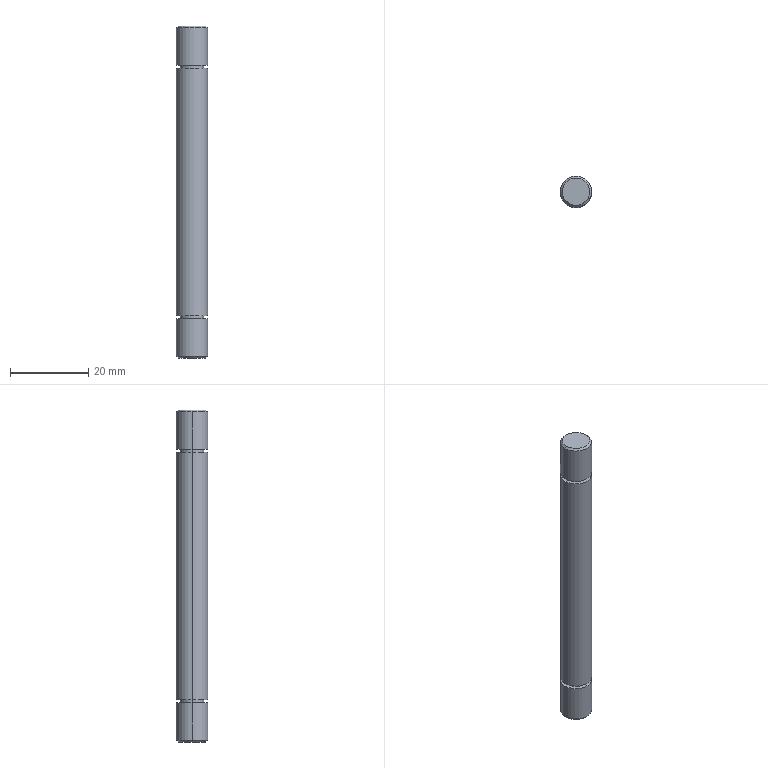Part | STEP file | 8XS200020 | 1 solid | 20 faces | box 8 x 8 x 85 mm | volume 4231 mm3 | cylinder 10 | plane 6 | cone 4 | commonest cylinder face diameters 8 x6 6 x4
STEP:
#1=CARTESIAN_POINT('',(0.,0.,0.));
#2=DIRECTION('',(0.,0.,1.));
#3=DIRECTION('',(1.,0.,0.));
#4=AXIS2_PLACEMENT_3D('',#1,#2,#3);
#5=CARTESIAN_POINT('',(3.5,0.,85.));
#6=VERTEX_POINT('',#5);
#7=CARTESIAN_POINT('',(-3.5,0.,85.));
#8=VERTEX_POINT('',#7);
#9=CARTESIAN_POINT('',(0.,0.,85.));
#10=DIRECTION('',(0.,0.,1.));
#11=DIRECTION('',(1.,0.,0.));
#12=AXIS2_PLACEMENT_3D('',#9,#10,#11);
#13=CIRCLE('',#12,3.5);
#14=CARTESIAN_POINT('',(0.,0.,85.));
#15=DIRECTION('',(0.,0.,-1.));
#16=DIRECTION('',(-1.,0.,0.));
#17=AXIS2_PLACEMENT_3D('',#14,#15,#16);
#18=CONICAL_SURFACE('',#17,3.5,0.7854);
#19=CARTESIAN_POINT('',(3.142,0.));
#20=DIRECTION('',(-1.,0.));
#21=VECTOR('',#20,1.);
#22=LINE('',#19,#21);
#23=(GEOMETRIC_REPRESENTATION_CONTEXT(2)PARAMETRIC_REPRESENTATION_CONTEXT()REPRESENTATION_CONTEXT('',''));
#24=DEFINITIONAL_REPRESENTATION('',(#22),#23);
#25=PCURVE('',#18,#24);
#26=CARTESIAN_POINT('',(0.,0.,85.));
#27=DIRECTION('',(0.,0.,1.));
#28=DIRECTION('',(1.,0.,0.));
#29=AXIS2_PLACEMENT_3D('',#26,#27,#28);
#30=PLANE('',#29);
#31=CARTESIAN_POINT('',(0.,0.));
#32=DIRECTION('',(1.,0.));
#33=AXIS2_PLACEMENT_2D('',#31,#32);
#34=CIRCLE('',#33,3.5);
#35=(GEOMETRIC_REPRESENTATION_CONTEXT(2)PARAMETRIC_REPRESENTATION_CONTEXT()REPRESENTATION_CONTEXT('',''));
#36=DEFINITIONAL_REPRESENTATION('',(#34),#35);
#37=PCURVE('',#30,#36);
#38=SURFACE_CURVE('',#13,(#25,#37),.PCURVE_S1.);
#39=EDGE_CURVE('',#6,#8,#38,.T.);
#40=ORIENTED_EDGE('',*,*,#39,.F.);
#41=CARTESIAN_POINT('',(4.,0.,84.5));
#42=VERTEX_POINT('',#41);
#43=CARTESIAN_POINT('',(3.5,0.,85.));
#44=DIRECTION('',(0.7071,0.,-0.7071));
#45=VECTOR('',#44,1.);
#46=LINE('',#43,#45);
#47=CARTESIAN_POINT('',(3.142,0.));
#48=DIRECTION('',(0.,1.));
#49=VECTOR('',#48,1.);
#50=LINE('',#47,#49);
#51=(GEOMETRIC_REPRESENTATION_CONTEXT(2)PARAMETRIC_REPRESENTATION_CONTEXT()REPRESENTATION_CONTEXT('',''));
#52=DEFINITIONAL_REPRESENTATION('',(#50),#51);
#53=PCURVE('',#18,#52);
#54=CARTESIAN_POINT('',(0.,0.,85.));
#55=DIRECTION('',(0.,0.,-1.));
#56=DIRECTION('',(-1.,0.,0.));
#57=AXIS2_PLACEMENT_3D('',#54,#55,#56);
#58=CONICAL_SURFACE('',#57,3.5,0.7854);
#59=CARTESIAN_POINT('',(3.142,0.));
#60=DIRECTION('',(0.,1.));
#61=VECTOR('',#60,1.);
#62=LINE('',#59,#61);
#63=(GEOMETRIC_REPRESENTATION_CONTEXT(2)PARAMETRIC_REPRESENTATION_CONTEXT()REPRESENTATION_CONTEXT('',''));
#64=DEFINITIONAL_REPRESENTATION('',(#62),#63);
#65=PCURVE('',#58,#64);
#66=SURFACE_CURVE('',#46,(#53,#65),.PCURVE_S1.);
#67=EDGE_CURVE('',#6,#42,#66,.T.);
#68=ORIENTED_EDGE('',*,*,#67,.T.);
#69=CARTESIAN_POINT('',(-4.,0.,84.5));
#70=VERTEX_POINT('',#69);
#71=CARTESIAN_POINT('',(0.,0.,84.5));
#72=DIRECTION('',(0.,0.,-1.));
#73=DIRECTION('',(1.,0.,0.));
#74=AXIS2_PLACEMENT_3D('',#71,#72,#73);
#75=CIRCLE('',#74,4.);
#76=CARTESIAN_POINT('',(-3.142,0.5));
#77=DIRECTION('',(1.,0.));
#78=VECTOR('',#77,1.);
#79=LINE('',#76,#78);
#80=(GEOMETRIC_REPRESENTATION_CONTEXT(2)PARAMETRIC_REPRESENTATION_CONTEXT()REPRESENTATION_CONTEXT('',''));
#81=DEFINITIONAL_REPRESENTATION('',(#79),#80);
#82=PCURVE('',#18,#81);
#83=CARTESIAN_POINT('',(0.,0.,85.));
#84=DIRECTION('',(0.,0.,-1.));
#85=DIRECTION('',(-1.,0.,0.));
#86=AXIS2_PLACEMENT_3D('',#83,#84,#85);
#87=CYLINDRICAL_SURFACE('',#86,4.);
#88=CARTESIAN_POINT('',(-3.142,0.5));
#89=DIRECTION('',(1.,0.));
#90=VECTOR('',#89,1.);
#91=LINE('',#88,#90);
#92=(GEOMETRIC_REPRESENTATION_CONTEXT(2)PARAMETRIC_REPRESENTATION_CONTEXT()REPRESENTATION_CONTEXT('',''));
#93=DEFINITIONAL_REPRESENTATION('',(#91),#92);
#94=PCURVE('',#87,#93);
#95=SURFACE_CURVE('',#75,(#82,#94),.PCURVE_S1.);
#96=EDGE_CURVE('',#70,#42,#95,.T.);
#97=ORIENTED_EDGE('',*,*,#96,.F.);
#98=CARTESIAN_POINT('',(-3.5,0.,85.));
#99=DIRECTION('',(-0.7071,0.,-0.7071));
#100=VECTOR('',#99,1.);
#101=LINE('',#98,#100);
#102=CARTESIAN_POINT('',(0.,0.));
#103=DIRECTION('',(0.,1.));
#104=VECTOR('',#103,1.);
#105=LINE('',#102,#104);
#106=(GEOMETRIC_REPRESENTATION_CONTEXT(2)PARAMETRIC_REPRESENTATION_CONTEXT()REPRESENTATION_CONTEXT('',''));
#107=DEFINITIONAL_REPRESENTATION('',(#105),#106);
#108=PCURVE('',#18,#107);
#109=CARTESIAN_POINT('',(6.283,0.));
#110=DIRECTION('',(0.,1.));
#111=VECTOR('',#110,1.);
#112=LINE('',#109,#111);
#113=(GEOMETRIC_REPRESENTATION_CONTEXT(2)PARAMETRIC_REPRESENTATION_CONTEXT()REPRESENTATION_CONTEXT('',''));
#114=DEFINITIONAL_REPRESENTATION('',(#112),#113);
#115=PCURVE('',#58,#114);
#116=SURFACE_CURVE('',#101,(#108,#115),.PCURVE_S1.);
#117=EDGE_CURVE('',#8,#70,#116,.T.);
#118=ORIENTED_EDGE('',*,*,#117,.F.);
#119=EDGE_LOOP('',(#40,#68,#97,#118));
#120=FACE_BOUND('',#119,.T.);
#121=ADVANCED_FACE('',(#120),#18,.T.);
#122=CARTESIAN_POINT('',(-3.5,0.,0.));
#123=VERTEX_POINT('',#122);
#124=CARTESIAN_POINT('',(3.5,0.,0.));
#125=VERTEX_POINT('',#124);
#126=CARTESIAN_POINT('',(0.,0.,0.));
#127=DIRECTION('',(0.,0.,-1.));
#128=DIRECTION('',(1.,0.,0.));
#129=AXIS2_PLACEMENT_3D('',#126,#127,#128);
#130=CIRCLE('',#129,3.5);
#131=CARTESIAN_POINT('',(0.,0.,0.5));
#132=DIRECTION('',(0.,0.,1.));
#133=DIRECTION('',(1.,0.,0.));
#134=AXIS2_PLACEMENT_3D('',#131,#132,#133);
#135=CONICAL_SURFACE('',#134,4.,0.7854);
#136=CARTESIAN_POINT('',(6.283,-0.5));
#137=DIRECTION('',(-1.,0.));
#138=VECTOR('',#137,1.);
#139=LINE('',#136,#138);
#140=(GEOMETRIC_REPRESENTATION_CONTEXT(2)PARAMETRIC_REPRESENTATION_CONTEXT()REPRESENTATION_CONTEXT('',''));
#141=DEFINITIONAL_REPRESENTATION('',(#139),#140);
#142=PCURVE('',#135,#141);
#143=CARTESIAN_POINT('',(0.,0.,0.));
#144=DIRECTION('',(0.,0.,1.));
#145=DIRECTION('',(1.,0.,0.));
#146=AXIS2_PLACEMENT_3D('',#143,#144,#145);
#147=PLANE('',#146);
#148=CARTESIAN_POINT('',(3.5,0.));
#149=CARTESIAN_POINT('',(3.5,-6.062));
#150=CARTESIAN_POINT('',(-1.75,-3.031));
#151=CARTESIAN_POINT('',(-7.,0.));
#152=CARTESIAN_POINT('',(-1.75,3.031));
#153=CARTESIAN_POINT('',(3.5,6.062));
#154=CARTESIAN_POINT('',(3.5,0.));
#155=(BOUNDED_CURVE()B_SPLINE_CURVE(2,(#148,#149,#150,#151,#152,#153,#154),.UNSPECIFIED.,.T.,.F.)B_SPLINE_CURVE_WITH_KNOTS((1,2,2,2,2,1),(-2.094,0.,2.094,4.189,6.283,8.378),.UNSPECIFIED.)CURVE()GEOMETRIC_REPRESENTATION_ITEM()RATIONAL_B_SPLINE_CURVE((1.,0.5,1.,0.5,1.,0.5,1.))REPRESENTATION_ITEM(''));
#156=(GEOMETRIC_REPRESENTATION_CONTEXT(2)PARAMETRIC_REPRESENTATION_CONTEXT()REPRESENTATION_CONTEXT('',''));
#157=DEFINITIONAL_REPRESENTATION('',(#155),#156);
#158=PCURVE('',#147,#157);
#159=SURFACE_CURVE('',#130,(#142,#158),.PCURVE_S1.);
#160=EDGE_CURVE('',#123,#125,#159,.T.);
#161=ORIENTED_EDGE('',*,*,#160,.F.);
#162=CARTESIAN_POINT('',(-4.,0.,0.5));
#163=VERTEX_POINT('',#162);
#164=CARTESIAN_POINT('',(-4.,0.,0.5));
#165=DIRECTION('',(-0.7071,0.,0.7071));
#166=VECTOR('',#165,1.);
#167=LINE('',#164,#166);
#168=CARTESIAN_POINT('',(3.142,0.));
#169=DIRECTION('',(0.,1.));
#170=VECTOR('',#169,1.);
#171=LINE('',#168,#170);
#172=(GEOMETRIC_REPRESENTATION_CONTEXT(2)PARAMETRIC_REPRESENTATION_CONTEXT()REPRESENTATION_CONTEXT('',''));
#173=DEFINITIONAL_REPRESENTATION('',(#171),#172);
#174=PCURVE('',#135,#173);
#175=CARTESIAN_POINT('',(0.,0.,0.5));
#176=DIRECTION('',(0.,0.,1.));
#177=DIRECTION('',(1.,0.,0.));
#178=AXIS2_PLACEMENT_3D('',#175,#176,#177);
#179=CONICAL_SURFACE('',#178,4.,0.7854);
#180=CARTESIAN_POINT('',(3.142,0.));
#181=DIRECTION('',(0.,1.));
#182=VECTOR('',#181,1.);
#183=LINE('',#180,#182);
#184=(GEOMETRIC_REPRESENTATION_CONTEXT(2)PARAMETRIC_REPRESENTATION_CONTEXT()REPRESENTATION_CONTEXT('',''));
#185=DEFINITIONAL_REPRESENTATION('',(#183),#184);
#186=PCURVE('',#179,#185);
#187=SURFACE_CURVE('',#167,(#174,#186),.PCURVE_S1.);
#188=EDGE_CURVE('',#123,#163,#187,.T.);
#189=ORIENTED_EDGE('',*,*,#188,.T.);
#190=CARTESIAN_POINT('',(4.,0.,0.5));
#191=VERTEX_POINT('',#190);
#192=CARTESIAN_POINT('',(0.,0.,0.5));
#193=DIRECTION('',(0.,0.,1.));
#194=DIRECTION('',(1.,0.,0.));
#195=AXIS2_PLACEMENT_3D('',#192,#193,#194);
#196=CIRCLE('',#195,4.);
#197=CARTESIAN_POINT('',(0.,0.));
#198=DIRECTION('',(1.,0.));
#199=VECTOR('',#198,1.);
#200=LINE('',#197,#199);
#201=(GEOMETRIC_REPRESENTATION_CONTEXT(2)PARAMETRIC_REPRESENTATION_CONTEXT()REPRESENTATION_CONTEXT('',''));
#202=DEFINITIONAL_REPRESENTATION('',(#200),#201);
#203=PCURVE('',#135,#202);
#204=CARTESIAN_POINT('',(0.,0.,10.));
#205=DIRECTION('',(0.,0.,-1.));
#206=DIRECTION('',(-1.,0.,0.));
#207=AXIS2_PLACEMENT_3D('',#204,#205,#206);
#208=CYLINDRICAL_SURFACE('',#207,4.);
#209=CARTESIAN_POINT('',(3.142,9.5));
#210=DIRECTION('',(-1.,0.));
#211=VECTOR('',#210,1.);
#212=LINE('',#209,#211);
#213=(GEOMETRIC_REPRESENTATION_CONTEXT(2)PARAMETRIC_REPRESENTATION_CONTEXT()REPRESENTATION_CONTEXT('',''));
#214=DEFINITIONAL_REPRESENTATION('',(#212),#213);
#215=PCURVE('',#208,#214);
#216=SURFACE_CURVE('',#196,(#203,#215),.PCURVE_S1.);
#217=EDGE_CURVE('',#191,#163,#216,.T.);
#218=ORIENTED_EDGE('',*,*,#217,.F.);
#219=CARTESIAN_POINT('',(4.,0.,0.5));
#220=DIRECTION('',(0.7071,0.,0.7071));
#221=VECTOR('',#220,1.);
#222=LINE('',#219,#221);
#223=CARTESIAN_POINT('',(0.,0.));
#224=DIRECTION('',(0.,1.));
#225=VECTOR('',#224,1.);
#226=LINE('',#223,#225);
#227=(GEOMETRIC_REPRESENTATION_CONTEXT(2)PARAMETRIC_REPRESENTATION_CONTEXT()REPRESENTATION_CONTEXT('',''));
#228=DEFINITIONAL_REPRESENTATION('',(#226),#227);
#229=PCURVE('',#135,#228);
#230=CARTESIAN_POINT('',(6.283,0.));
#231=DIRECTION('',(0.,1.));
#232=VECTOR('',#231,1.);
#233=LINE('',#230,#232);
#234=(GEOMETRIC_REPRESENTATION_CONTEXT(2)PARAMETRIC_REPRESENTATION_CONTEXT()REPRESENTATION_CONTEXT('',''));
#235=DEFINITIONAL_REPRESENTATION('',(#233),#234);
#236=PCURVE('',#179,#235);
#237=SURFACE_CURVE('',#222,(#229,#236),.PCURVE_S1.);
#238=EDGE_CURVE('',#125,#191,#237,.T.);
#239=ORIENTED_EDGE('',*,*,#238,.F.);
#240=EDGE_LOOP('',(#161,#189,#218,#239));
#241=FACE_BOUND('',#240,.T.);
#242=ADVANCED_FACE('',(#241),#135,.T.);
#243=ORIENTED_EDGE('',*,*,#96,.T.);
#244=CARTESIAN_POINT('',(4.,0.,75.));
#245=VERTEX_POINT('',#244);
#246=CARTESIAN_POINT('',(4.,0.,85.));
#247=DIRECTION('',(0.,0.,-1.));
#248=VECTOR('',#247,1.);
#249=LINE('',#246,#248);
#250=CARTESIAN_POINT('',(3.142,0.));
#251=DIRECTION('',(0.,1.));
#252=VECTOR('',#251,1.);
#253=LINE('',#250,#252);
#254=(GEOMETRIC_REPRESENTATION_CONTEXT(2)PARAMETRIC_REPRESENTATION_CONTEXT()REPRESENTATION_CONTEXT('',''));
#255=DEFINITIONAL_REPRESENTATION('',(#253),#254);
#256=PCURVE('',#87,#255);
#257=CARTESIAN_POINT('',(0.,0.,85.));
#258=DIRECTION('',(0.,0.,-1.));
#259=DIRECTION('',(-1.,0.,0.));
#260=AXIS2_PLACEMENT_3D('',#257,#258,#259);
#261=CYLINDRICAL_SURFACE('',#260,4.);
#262=CARTESIAN_POINT('',(3.142,0.));
#263=DIRECTION('',(0.,1.));
#264=VECTOR('',#263,1.);
#265=LINE('',#262,#264);
#266=(GEOMETRIC_REPRESENTATION_CONTEXT(2)PARAMETRIC_REPRESENTATION_CONTEXT()REPRESENTATION_CONTEXT('',''));
#267=DEFINITIONAL_REPRESENTATION('',(#265),#266);
#268=PCURVE('',#261,#267);
#269=SURFACE_CURVE('',#249,(#256,#268),.PCURVE_S1.);
#270=EDGE_CURVE('',#42,#245,#269,.T.);
#271=ORIENTED_EDGE('',*,*,#270,.T.);
#272=CARTESIAN_POINT('',(-4.,0.,75.));
#273=VERTEX_POINT('',#272);
#274=CARTESIAN_POINT('',(0.,0.,75.));
#275=DIRECTION('',(0.,0.,1.));
#276=DIRECTION('',(1.,0.,0.));
#277=AXIS2_PLACEMENT_3D('',#274,#275,#276);
#278=CIRCLE('',#277,4.);
#279=CARTESIAN_POINT('',(3.142,10.));
#280=DIRECTION('',(-1.,0.));
#281=VECTOR('',#280,1.);
#282=LINE('',#279,#281);
#283=(GEOMETRIC_REPRESENTATION_CONTEXT(2)PARAMETRIC_REPRESENTATION_CONTEXT()REPRESENTATION_CONTEXT('',''));
#284=DEFINITIONAL_REPRESENTATION('',(#282),#283);
#285=PCURVE('',#87,#284);
#286=CARTESIAN_POINT('',(0.,0.,75.));
#287=DIRECTION('',(0.,0.,1.));
#288=DIRECTION('',(1.,0.,0.));
#289=AXIS2_PLACEMENT_3D('',#286,#287,#288);
#290=PLANE('',#289);
#291=CARTESIAN_POINT('',(0.,0.));
#292=DIRECTION('',(1.,0.));
#293=AXIS2_PLACEMENT_2D('',#291,#292);
#294=CIRCLE('',#293,4.);
#295=(GEOMETRIC_REPRESENTATION_CONTEXT(2)PARAMETRIC_REPRESENTATION_CONTEXT()REPRESENTATION_CONTEXT('',''));
#296=DEFINITIONAL_REPRESENTATION('',(#294),#295);
#297=PCURVE('',#290,#296);
#298=SURFACE_CURVE('',#278,(#285,#297),.PCURVE_S1.);
#299=EDGE_CURVE('',#245,#273,#298,.T.);
#300=ORIENTED_EDGE('',*,*,#299,.T.);
#301=CARTESIAN_POINT('',(-4.,0.,85.));
#302=DIRECTION('',(0.,0.,-1.));
#303=VECTOR('',#302,1.);
#304=LINE('',#301,#303);
#305=CARTESIAN_POINT('',(0.,0.));
#306=DIRECTION('',(0.,1.));
#307=VECTOR('',#306,1.);
#308=LINE('',#305,#307);
#309=(GEOMETRIC_REPRESENTATION_CONTEXT(2)PARAMETRIC_REPRESENTATION_CONTEXT()REPRESENTATION_CONTEXT('',''));
#310=DEFINITIONAL_REPRESENTATION('',(#308),#309);
#311=PCURVE('',#87,#310);
#312=CARTESIAN_POINT('',(6.283,0.));
#313=DIRECTION('',(0.,1.));
#314=VECTOR('',#313,1.);
#315=LINE('',#312,#314);
#316=(GEOMETRIC_REPRESENTATION_CONTEXT(2)PARAMETRIC_REPRESENTATION_CONTEXT()REPRESENTATION_CONTEXT('',''));
#317=DEFINITIONAL_REPRESENTATION('',(#315),#316);
#318=PCURVE('',#261,#317);
#319=SURFACE_CURVE('',#304,(#311,#318),.PCURVE_S1.);
#320=EDGE_CURVE('',#70,#273,#319,.T.);
#321=ORIENTED_EDGE('',*,*,#320,.F.);
#322=EDGE_LOOP('',(#243,#271,#300,#321));
#323=FACE_BOUND('',#322,.T.);
#324=ADVANCED_FACE('',(#323),#87,.T.);
#325=CARTESIAN_POINT('',(3.,0.,75.));
#326=VERTEX_POINT('',#325);
#327=CARTESIAN_POINT('',(-3.,0.,75.));
#328=VERTEX_POINT('',#327);
#329=CARTESIAN_POINT('',(0.,0.,75.));
#330=DIRECTION('',(0.,0.,1.));
#331=DIRECTION('',(1.,0.,0.));
#332=AXIS2_PLACEMENT_3D('',#329,#330,#331);
#333=CIRCLE('',#332,3.);
#334=CARTESIAN_POINT('',(0.,0.,75.));
#335=DIRECTION('',(0.,0.,-1.));
#336=DIRECTION('',(-1.,0.,0.));
#337=AXIS2_PLACEMENT_3D('',#334,#335,#336);
#338=CYLINDRICAL_SURFACE('',#337,3.);
#339=CARTESIAN_POINT('',(3.142,0.));
#340=DIRECTION('',(-1.,0.));
#341=VECTOR('',#340,1.);
#342=LINE('',#339,#341);
#343=(GEOMETRIC_REPRESENTATION_CONTEXT(2)PARAMETRIC_REPRESENTATION_CONTEXT()REPRESENTATION_CONTEXT('',''));
#344=DEFINITIONAL_REPRESENTATION('',(#342),#343);
#345=PCURVE('',#338,#344);
#346=CARTESIAN_POINT('',(0.,0.));
#347=DIRECTION('',(1.,0.));
#348=AXIS2_PLACEMENT_2D('',#346,#347);
#349=CIRCLE('',#348,3.);
#350=(GEOMETRIC_REPRESENTATION_CONTEXT(2)PARAMETRIC_REPRESENTATION_CONTEXT()REPRESENTATION_CONTEXT('',''));
#351=DEFINITIONAL_REPRESENTATION('',(#349),#350);
#352=PCURVE('',#290,#351);
#353=SURFACE_CURVE('',#333,(#345,#352),.PCURVE_S1.);
#354=EDGE_CURVE('',#326,#328,#353,.T.);
#355=ORIENTED_EDGE('',*,*,#354,.F.);
#356=CARTESIAN_POINT('',(3.,0.,74.2));
#357=VERTEX_POINT('',#356);
#358=CARTESIAN_POINT('',(3.,0.,75.));
#359=DIRECTION('',(0.,0.,-1.));
#360=VECTOR('',#359,1.);
#361=LINE('',#358,#360);
#362=CARTESIAN_POINT('',(3.142,0.));
#363=DIRECTION('',(0.,1.));
#364=VECTOR('',#363,1.);
#365=LINE('',#362,#364);
#366=(GEOMETRIC_REPRESENTATION_CONTEXT(2)PARAMETRIC_REPRESENTATION_CONTEXT()REPRESENTATION_CONTEXT('',''));
#367=DEFINITIONAL_REPRESENTATION('',(#365),#366);
#368=PCURVE('',#338,#367);
#369=CARTESIAN_POINT('',(0.,0.,75.));
#370=DIRECTION('',(0.,0.,-1.));
#371=DIRECTION('',(-1.,0.,0.));
#372=AXIS2_PLACEMENT_3D('',#369,#370,#371);
#373=CYLINDRICAL_SURFACE('',#372,3.);
#374=CARTESIAN_POINT('',(3.142,0.));
#375=DIRECTION('',(0.,1.));
#376=VECTOR('',#375,1.);
#377=LINE('',#374,#376);
#378=(GEOMETRIC_REPRESENTATION_CONTEXT(2)PARAMETRIC_REPRESENTATION_CONTEXT()REPRESENTATION_CONTEXT('',''));
#379=DEFINITIONAL_REPRESENTATION('',(#377),#378);
#380=PCURVE('',#373,#379);
#381=SURFACE_CURVE('',#361,(#368,#380),.PCURVE_S1.);
#382=EDGE_CURVE('',#326,#357,#381,.T.);
#383=ORIENTED_EDGE('',*,*,#382,.T.);
#384=CARTESIAN_POINT('',(-3.,0.,74.2));
#385=VERTEX_POINT('',#384);
#386=CARTESIAN_POINT('',(0.,0.,74.2));
#387=DIRECTION('',(0.,0.,1.));
#388=DIRECTION('',(1.,0.,0.));
#389=AXIS2_PLACEMENT_3D('',#386,#387,#388);
#390=CIRCLE('',#389,3.);
#391=CARTESIAN_POINT('',(3.142,0.8));
#392=DIRECTION('',(-1.,0.));
#393=VECTOR('',#392,1.);
#394=LINE('',#391,#393);
#395=(GEOMETRIC_REPRESENTATION_CONTEXT(2)PARAMETRIC_REPRESENTATION_CONTEXT()REPRESENTATION_CONTEXT('',''));
#396=DEFINITIONAL_REPRESENTATION('',(#394),#395);
#397=PCURVE('',#338,#396);
#398=CARTESIAN_POINT('',(0.,0.,74.2));
#399=DIRECTION('',(0.,0.,1.));
#400=DIRECTION('',(1.,0.,0.));
#401=AXIS2_PLACEMENT_3D('',#398,#399,#400);
#402=PLANE('',#401);
#403=CARTESIAN_POINT('',(0.,0.));
#404=DIRECTION('',(1.,0.));
#405=AXIS2_PLACEMENT_2D('',#403,#404);
#406=CIRCLE('',#405,3.);
#407=(GEOMETRIC_REPRESENTATION_CONTEXT(2)PARAMETRIC_REPRESENTATION_CONTEXT()REPRESENTATION_CONTEXT('',''));
#408=DEFINITIONAL_REPRESENTATION('',(#406),#407);
#409=PCURVE('',#402,#408);
#410=SURFACE_CURVE('',#390,(#397,#409),.PCURVE_S1.);
#411=EDGE_CURVE('',#357,#385,#410,.T.);
#412=ORIENTED_EDGE('',*,*,#411,.T.);
#413=CARTESIAN_POINT('',(-3.,0.,75.));
#414=DIRECTION('',(0.,0.,-1.));
#415=VECTOR('',#414,1.);
#416=LINE('',#413,#415);
#417=CARTESIAN_POINT('',(0.,0.));
#418=DIRECTION('',(0.,1.));
#419=VECTOR('',#418,1.);
#420=LINE('',#417,#419);
#421=(GEOMETRIC_REPRESENTATION_CONTEXT(2)PARAMETRIC_REPRESENTATION_CONTEXT()REPRESENTATION_CONTEXT('',''));
#422=DEFINITIONAL_REPRESENTATION('',(#420),#421);
#423=PCURVE('',#338,#422);
#424=CARTESIAN_POINT('',(6.283,0.));
#425=DIRECTION('',(0.,1.));
#426=VECTOR('',#425,1.);
#427=LINE('',#424,#426);
#428=(GEOMETRIC_REPRESENTATION_CONTEXT(2)PARAMETRIC_REPRESENTATION_CONTEXT()REPRESENTATION_CONTEXT('',''));
#429=DEFINITIONAL_REPRESENTATION('',(#427),#428);
#430=PCURVE('',#373,#429);
#431=SURFACE_CURVE('',#416,(#423,#430),.PCURVE_S1.);
#432=EDGE_CURVE('',#328,#385,#431,.T.);
#433=ORIENTED_EDGE('',*,*,#432,.F.);
#434=EDGE_LOOP('',(#355,#383,#412,#433));
#435=FACE_BOUND('',#434,.T.);
#436=ADVANCED_FACE('',(#435),#338,.T.);
#437=CARTESIAN_POINT('',(4.,0.,74.2));
#438=VERTEX_POINT('',#437);
#439=CARTESIAN_POINT('',(-4.,0.,74.2));
#440=VERTEX_POINT('',#439);
#441=CARTESIAN_POINT('',(0.,0.,74.2));
#442=DIRECTION('',(0.,0.,1.));
#443=DIRECTION('',(1.,0.,0.));
#444=AXIS2_PLACEMENT_3D('',#441,#442,#443);
#445=CIRCLE('',#444,4.);
#446=CARTESIAN_POINT('',(0.,0.,74.2));
#447=DIRECTION('',(0.,0.,-1.));
#448=DIRECTION('',(-1.,0.,0.));
#449=AXIS2_PLACEMENT_3D('',#446,#447,#448);
#450=CYLINDRICAL_SURFACE('',#449,4.);
#451=CARTESIAN_POINT('',(3.142,0.));
#452=DIRECTION('',(-1.,0.));
#453=VECTOR('',#452,1.);
#454=LINE('',#451,#453);
#455=(GEOMETRIC_REPRESENTATION_CONTEXT(2)PARAMETRIC_REPRESENTATION_CONTEXT()REPRESENTATION_CONTEXT('',''));
#456=DEFINITIONAL_REPRESENTATION('',(#454),#455);
#457=PCURVE('',#450,#456);
#458=CARTESIAN_POINT('',(0.,0.));
#459=DIRECTION('',(1.,0.));
#460=AXIS2_PLACEMENT_2D('',#458,#459);
#461=CIRCLE('',#460,4.);
#462=(GEOMETRIC_REPRESENTATION_CONTEXT(2)PARAMETRIC_REPRESENTATION_CONTEXT()REPRESENTATION_CONTEXT('',''));
#463=DEFINITIONAL_REPRESENTATION('',(#461),#462);
#464=PCURVE('',#402,#463);
#465=SURFACE_CURVE('',#445,(#457,#464),.PCURVE_S1.);
#466=EDGE_CURVE('',#438,#440,#465,.T.);
#467=ORIENTED_EDGE('',*,*,#466,.F.);
#468=CARTESIAN_POINT('',(4.,0.,10.8));
#469=VERTEX_POINT('',#468);
#470=CARTESIAN_POINT('',(4.,0.,74.2));
#471=DIRECTION('',(0.,0.,-1.));
#472=VECTOR('',#471,1.);
#473=LINE('',#470,#472);
#474=CARTESIAN_POINT('',(3.142,0.));
#475=DIRECTION('',(0.,1.));
#476=VECTOR('',#475,1.);
#477=LINE('',#474,#476);
#478=(GEOMETRIC_REPRESENTATION_CONTEXT(2)PARAMETRIC_REPRESENTATION_CONTEXT()REPRESENTATION_CONTEXT('',''));
#479=DEFINITIONAL_REPRESENTATION('',(#477),#478);
#480=PCURVE('',#450,#479);
#481=CARTESIAN_POINT('',(0.,0.,74.2));
#482=DIRECTION('',(0.,0.,-1.));
#483=DIRECTION('',(-1.,0.,0.));
#484=AXIS2_PLACEMENT_3D('',#481,#482,#483);
#485=CYLINDRICAL_SURFACE('',#484,4.);
#486=CARTESIAN_POINT('',(3.142,0.));
#487=DIRECTION('',(0.,1.));
#488=VECTOR('',#487,1.);
#489=LINE('',#486,#488);
#490=(GEOMETRIC_REPRESENTATION_CONTEXT(2)PARAMETRIC_REPRESENTATION_CONTEXT()REPRESENTATION_CONTEXT('',''));
#491=DEFINITIONAL_REPRESENTATION('',(#489),#490);
#492=PCURVE('',#485,#491);
#493=SURFACE_CURVE('',#473,(#480,#492),.PCURVE_S1.);
#494=EDGE_CURVE('',#438,#469,#493,.T.);
#495=ORIENTED_EDGE('',*,*,#494,.T.);
#496=CARTESIAN_POINT('',(-4.,0.,10.8));
#497=VERTEX_POINT('',#496);
#498=CARTESIAN_POINT('',(0.,0.,10.8));
#499=DIRECTION('',(0.,0.,1.));
#500=DIRECTION('',(1.,0.,0.));
#501=AXIS2_PLACEMENT_3D('',#498,#499,#500);
#502=CIRCLE('',#501,4.);
#503=CARTESIAN_POINT('',(3.142,63.4));
#504=DIRECTION('',(-1.,0.));
#505=VECTOR('',#504,1.);
#506=LINE('',#503,#505);
#507=(GEOMETRIC_REPRESENTATION_CONTEXT(2)PARAMETRIC_REPRESENTATION_CONTEXT()REPRESENTATION_CONTEXT('',''));
#508=DEFINITIONAL_REPRESENTATION('',(#506),#507);
#509=PCURVE('',#450,#508);
#510=CARTESIAN_POINT('',(0.,0.,10.8));
#511=DIRECTION('',(0.,0.,1.));
#512=DIRECTION('',(1.,0.,0.));
#513=AXIS2_PLACEMENT_3D('',#510,#511,#512);
#514=PLANE('',#513);
#515=CARTESIAN_POINT('',(0.,0.));
#516=DIRECTION('',(1.,0.));
#517=AXIS2_PLACEMENT_2D('',#515,#516);
#518=CIRCLE('',#517,4.);
#519=(GEOMETRIC_REPRESENTATION_CONTEXT(2)PARAMETRIC_REPRESENTATION_CONTEXT()REPRESENTATION_CONTEXT('',''));
#520=DEFINITIONAL_REPRESENTATION('',(#518),#519);
#521=PCURVE('',#514,#520);
#522=SURFACE_CURVE('',#502,(#509,#521),.PCURVE_S1.);
#523=EDGE_CURVE('',#469,#497,#522,.T.);
#524=ORIENTED_EDGE('',*,*,#523,.T.);
#525=CARTESIAN_POINT('',(-4.,0.,74.2));
#526=DIRECTION('',(0.,0.,-1.));
#527=VECTOR('',#526,1.);
#528=LINE('',#525,#527);
#529=CARTESIAN_POINT('',(0.,0.));
#530=DIRECTION('',(0.,1.));
#531=VECTOR('',#530,1.);
#532=LINE('',#529,#531);
#533=(GEOMETRIC_REPRESENTATION_CONTEXT(2)PARAMETRIC_REPRESENTATION_CONTEXT()REPRESENTATION_CONTEXT('',''));
#534=DEFINITIONAL_REPRESENTATION('',(#532),#533);
#535=PCURVE('',#450,#534);
#536=CARTESIAN_POINT('',(6.283,0.));
#537=DIRECTION('',(0.,1.));
#538=VECTOR('',#537,1.);
#539=LINE('',#536,#538);
#540=(GEOMETRIC_REPRESENTATION_CONTEXT(2)PARAMETRIC_REPRESENTATION_CONTEXT()REPRESENTATION_CONTEXT('',''));
#541=DEFINITIONAL_REPRESENTATION('',(#539),#540);
#542=PCURVE('',#485,#541);
#543=SURFACE_CURVE('',#528,(#535,#542),.PCURVE_S1.);
#544=EDGE_CURVE('',#440,#497,#543,.T.);
#545=ORIENTED_EDGE('',*,*,#544,.F.);
#546=EDGE_LOOP('',(#467,#495,#524,#545));
#547=FACE_BOUND('',#546,.T.);
#548=ADVANCED_FACE('',(#547),#450,.T.);
#549=CARTESIAN_POINT('',(3.,0.,10.8));
#550=VERTEX_POINT('',#549);
#551=CARTESIAN_POINT('',(-3.,0.,10.8));
#552=VERTEX_POINT('',#551);
#553=CARTESIAN_POINT('',(0.,0.,10.8));
#554=DIRECTION('',(0.,0.,1.));
#555=DIRECTION('',(1.,0.,0.));
#556=AXIS2_PLACEMENT_3D('',#553,#554,#555);
#557=CIRCLE('',#556,3.);
#558=CARTESIAN_POINT('',(0.,0.,10.8));
#559=DIRECTION('',(0.,0.,-1.));
#560=DIRECTION('',(-1.,0.,0.));
#561=AXIS2_PLACEMENT_3D('',#558,#559,#560);
#562=CYLINDRICAL_SURFACE('',#561,3.);
#563=CARTESIAN_POINT('',(3.142,0.));
#564=DIRECTION('',(-1.,0.));
#565=VECTOR('',#564,1.);
#566=LINE('',#563,#565);
#567=(GEOMETRIC_REPRESENTATION_CONTEXT(2)PARAMETRIC_REPRESENTATION_CONTEXT()REPRESENTATION_CONTEXT('',''));
#568=DEFINITIONAL_REPRESENTATION('',(#566),#567);
#569=PCURVE('',#562,#568);
#570=CARTESIAN_POINT('',(0.,0.));
#571=DIRECTION('',(1.,0.));
#572=AXIS2_PLACEMENT_2D('',#570,#571);
#573=CIRCLE('',#572,3.);
#574=(GEOMETRIC_REPRESENTATION_CONTEXT(2)PARAMETRIC_REPRESENTATION_CONTEXT()REPRESENTATION_CONTEXT('',''));
#575=DEFINITIONAL_REPRESENTATION('',(#573),#574);
#576=PCURVE('',#514,#575);
#577=SURFACE_CURVE('',#557,(#569,#576),.PCURVE_S1.);
#578=EDGE_CURVE('',#550,#552,#577,.T.);
#579=ORIENTED_EDGE('',*,*,#578,.F.);
#580=CARTESIAN_POINT('',(3.,0.,10.));
#581=VERTEX_POINT('',#580);
#582=CARTESIAN_POINT('',(3.,0.,10.8));
#583=DIRECTION('',(0.,0.,-1.));
#584=VECTOR('',#583,1.);
#585=LINE('',#582,#584);
#586=CARTESIAN_POINT('',(3.142,0.));
#587=DIRECTION('',(0.,1.));
#588=VECTOR('',#587,1.);
#589=LINE('',#586,#588);
#590=(GEOMETRIC_REPRESENTATION_CONTEXT(2)PARAMETRIC_REPRESENTATION_CONTEXT()REPRESENTATION_CONTEXT('',''));
#591=DEFINITIONAL_REPRESENTATION('',(#589),#590);
#592=PCURVE('',#562,#591);
#593=CARTESIAN_POINT('',(0.,0.,10.8));
#594=DIRECTION('',(0.,0.,-1.));
#595=DIRECTION('',(-1.,0.,0.));
#596=AXIS2_PLACEMENT_3D('',#593,#594,#595);
#597=CYLINDRICAL_SURFACE('',#596,3.);
#598=CARTESIAN_POINT('',(3.142,0.));
#599=DIRECTION('',(0.,1.));
#600=VECTOR('',#599,1.);
#601=LINE('',#598,#600);
#602=(GEOMETRIC_REPRESENTATION_CONTEXT(2)PARAMETRIC_REPRESENTATION_CONTEXT()REPRESENTATION_CONTEXT('',''));
#603=DEFINITIONAL_REPRESENTATION('',(#601),#602);
#604=PCURVE('',#597,#603);
#605=SURFACE_CURVE('',#585,(#592,#604),.PCURVE_S1.);
#606=EDGE_CURVE('',#550,#581,#605,.T.);
#607=ORIENTED_EDGE('',*,*,#606,.T.);
#608=CARTESIAN_POINT('',(-3.,0.,10.));
#609=VERTEX_POINT('',#608);
#610=CARTESIAN_POINT('',(0.,0.,10.));
#611=DIRECTION('',(0.,0.,1.));
#612=DIRECTION('',(1.,0.,0.));
#613=AXIS2_PLACEMENT_3D('',#610,#611,#612);
#614=CIRCLE('',#613,3.);
#615=CARTESIAN_POINT('',(3.142,0.8));
#616=DIRECTION('',(-1.,0.));
#617=VECTOR('',#616,1.);
#618=LINE('',#615,#617);
#619=(GEOMETRIC_REPRESENTATION_CONTEXT(2)PARAMETRIC_REPRESENTATION_CONTEXT()REPRESENTATION_CONTEXT('',''));
#620=DEFINITIONAL_REPRESENTATION('',(#618),#619);
#621=PCURVE('',#562,#620);
#622=CARTESIAN_POINT('',(0.,0.,10.));
#623=DIRECTION('',(0.,0.,1.));
#624=DIRECTION('',(1.,0.,0.));
#625=AXIS2_PLACEMENT_3D('',#622,#623,#624);
#626=PLANE('',#625);
#627=CARTESIAN_POINT('',(0.,0.));
#628=DIRECTION('',(1.,0.));
#629=AXIS2_PLACEMENT_2D('',#627,#628);
#630=CIRCLE('',#629,3.);
#631=(GEOMETRIC_REPRESENTATION_CONTEXT(2)PARAMETRIC_REPRESENTATION_CONTEXT()REPRESENTATION_CONTEXT('',''));
#632=DEFINITIONAL_REPRESENTATION('',(#630),#631);
#633=PCURVE('',#626,#632);
#634=SURFACE_CURVE('',#614,(#621,#633),.PCURVE_S1.);
#635=EDGE_CURVE('',#581,#609,#634,.T.);
#636=ORIENTED_EDGE('',*,*,#635,.T.);
#637=CARTESIAN_POINT('',(-3.,0.,10.8));
#638=DIRECTION('',(0.,0.,-1.));
#639=VECTOR('',#638,1.);
#640=LINE('',#637,#639);
#641=CARTESIAN_POINT('',(0.,0.));
#642=DIRECTION('',(0.,1.));
#643=VECTOR('',#642,1.);
#644=LINE('',#641,#643);
#645=(GEOMETRIC_REPRESENTATION_CONTEXT(2)PARAMETRIC_REPRESENTATION_CONTEXT()REPRESENTATION_CONTEXT('',''));
#646=DEFINITIONAL_REPRESENTATION('',(#644),#645);
#647=PCURVE('',#562,#646);
#648=CARTESIAN_POINT('',(6.283,0.));
#649=DIRECTION('',(0.,1.));
#650=VECTOR('',#649,1.);
#651=LINE('',#648,#650);
#652=(GEOMETRIC_REPRESENTATION_CONTEXT(2)PARAMETRIC_REPRESENTATION_CONTEXT()REPRESENTATION_CONTEXT('',''));
#653=DEFINITIONAL_REPRESENTATION('',(#651),#652);
#654=PCURVE('',#597,#653);
#655=SURFACE_CURVE('',#640,(#647,#654),.PCURVE_S1.);
#656=EDGE_CURVE('',#552,#609,#655,.T.);
#657=ORIENTED_EDGE('',*,*,#656,.F.);
#658=EDGE_LOOP('',(#579,#607,#636,#657));
#659=FACE_BOUND('',#658,.T.);
#660=ADVANCED_FACE('',(#659),#562,.T.);
#661=CARTESIAN_POINT('',(4.,0.,10.));
#662=VERTEX_POINT('',#661);
#663=CARTESIAN_POINT('',(-4.,0.,10.));
#664=VERTEX_POINT('',#663);
#665=CARTESIAN_POINT('',(0.,0.,10.));
#666=DIRECTION('',(0.,0.,1.));
#667=DIRECTION('',(1.,0.,0.));
#668=AXIS2_PLACEMENT_3D('',#665,#666,#667);
#669=CIRCLE('',#668,4.);
#670=CARTESIAN_POINT('',(3.142,0.));
#671=DIRECTION('',(-1.,0.));
#672=VECTOR('',#671,1.);
#673=LINE('',#670,#672);
#674=(GEOMETRIC_REPRESENTATION_CONTEXT(2)PARAMETRIC_REPRESENTATION_CONTEXT()REPRESENTATION_CONTEXT('',''));
#675=DEFINITIONAL_REPRESENTATION('',(#673),#674);
#676=PCURVE('',#208,#675);
#677=CARTESIAN_POINT('',(0.,0.));
#678=DIRECTION('',(1.,0.));
#679=AXIS2_PLACEMENT_2D('',#677,#678);
#680=CIRCLE('',#679,4.);
#681=(GEOMETRIC_REPRESENTATION_CONTEXT(2)PARAMETRIC_REPRESENTATION_CONTEXT()REPRESENTATION_CONTEXT('',''));
#682=DEFINITIONAL_REPRESENTATION('',(#680),#681);
#683=PCURVE('',#626,#682);
#684=SURFACE_CURVE('',#669,(#676,#683),.PCURVE_S1.);
#685=EDGE_CURVE('',#662,#664,#684,.T.);
#686=ORIENTED_EDGE('',*,*,#685,.F.);
#687=CARTESIAN_POINT('',(4.,0.,10.));
#688=DIRECTION('',(0.,0.,-1.));
#689=VECTOR('',#688,1.);
#690=LINE('',#687,#689);
#691=CARTESIAN_POINT('',(3.142,0.));
#692=DIRECTION('',(0.,1.));
#693=VECTOR('',#692,1.);
#694=LINE('',#691,#693);
#695=(GEOMETRIC_REPRESENTATION_CONTEXT(2)PARAMETRIC_REPRESENTATION_CONTEXT()REPRESENTATION_CONTEXT('',''));
#696=DEFINITIONAL_REPRESENTATION('',(#694),#695);
#697=PCURVE('',#208,#696);
#698=CARTESIAN_POINT('',(0.,0.,10.));
#699=DIRECTION('',(0.,0.,-1.));
#700=DIRECTION('',(-1.,0.,0.));
#701=AXIS2_PLACEMENT_3D('',#698,#699,#700);
#702=CYLINDRICAL_SURFACE('',#701,4.);
#703=CARTESIAN_POINT('',(3.142,0.));
#704=DIRECTION('',(0.,1.));
#705=VECTOR('',#704,1.);
#706=LINE('',#703,#705);
#707=(GEOMETRIC_REPRESENTATION_CONTEXT(2)PARAMETRIC_REPRESENTATION_CONTEXT()REPRESENTATION_CONTEXT('',''));
#708=DEFINITIONAL_REPRESENTATION('',(#706),#707);
#709=PCURVE('',#702,#708);
#710=SURFACE_CURVE('',#690,(#697,#709),.PCURVE_S1.);
#711=EDGE_CURVE('',#662,#191,#710,.T.);
#712=ORIENTED_EDGE('',*,*,#711,.T.);
#713=ORIENTED_EDGE('',*,*,#217,.T.);
#714=CARTESIAN_POINT('',(-4.,0.,10.));
#715=DIRECTION('',(0.,0.,-1.));
#716=VECTOR('',#715,1.);
#717=LINE('',#714,#716);
#718=CARTESIAN_POINT('',(0.,0.));
#719=DIRECTION('',(0.,1.));
#720=VECTOR('',#719,1.);
#721=LINE('',#718,#720);
#722=(GEOMETRIC_REPRESENTATION_CONTEXT(2)PARAMETRIC_REPRESENTATION_CONTEXT()REPRESENTATION_CONTEXT('',''));
#723=DEFINITIONAL_REPRESENTATION('',(#721),#722);
#724=PCURVE('',#208,#723);
#725=CARTESIAN_POINT('',(6.283,0.));
#726=DIRECTION('',(0.,1.));
#727=VECTOR('',#726,1.);
#728=LINE('',#725,#727);
#729=(GEOMETRIC_REPRESENTATION_CONTEXT(2)PARAMETRIC_REPRESENTATION_CONTEXT()REPRESENTATION_CONTEXT('',''));
#730=DEFINITIONAL_REPRESENTATION('',(#728),#729);
#731=PCURVE('',#702,#730);
#732=SURFACE_CURVE('',#717,(#724,#731),.PCURVE_S1.);
#733=EDGE_CURVE('',#664,#163,#732,.T.);
#734=ORIENTED_EDGE('',*,*,#733,.F.);
#735=EDGE_LOOP('',(#686,#712,#713,#734));
#736=FACE_BOUND('',#735,.T.);
#737=ADVANCED_FACE('',(#736),#208,.T.);
#738=CARTESIAN_POINT('',(0.,0.,74.2));
#739=DIRECTION('',(0.,0.,1.));
#740=DIRECTION('',(1.,0.,0.));
#741=AXIS2_PLACEMENT_3D('',#738,#739,#740);
#742=CIRCLE('',#741,4.);
#743=CARTESIAN_POINT('',(0.,0.));
#744=DIRECTION('',(1.,0.));
#745=AXIS2_PLACEMENT_2D('',#743,#744);
#746=CIRCLE('',#745,4.);
#747=(GEOMETRIC_REPRESENTATION_CONTEXT(2)PARAMETRIC_REPRESENTATION_CONTEXT()REPRESENTATION_CONTEXT('',''));
#748=DEFINITIONAL_REPRESENTATION('',(#746),#747);
#749=PCURVE('',#402,#748);
#750=CARTESIAN_POINT('',(9.425,0.));
#751=DIRECTION('',(-1.,0.));
#752=VECTOR('',#751,1.);
#753=LINE('',#750,#752);
#754=(GEOMETRIC_REPRESENTATION_CONTEXT(2)PARAMETRIC_REPRESENTATION_CONTEXT()REPRESENTATION_CONTEXT('',''));
#755=DEFINITIONAL_REPRESENTATION('',(#753),#754);
#756=PCURVE('',#485,#755);
#757=SURFACE_CURVE('',#742,(#749,#756),.PCURVE_S1.);
#758=EDGE_CURVE('',#440,#438,#757,.T.);
#759=ORIENTED_EDGE('',*,*,#758,.T.);
#760=ORIENTED_EDGE('',*,*,#466,.T.);
#761=EDGE_LOOP('',(#759,#760));
#762=FACE_BOUND('',#761,.T.);
#763=CARTESIAN_POINT('',(0.,0.,74.2));
#764=DIRECTION('',(0.,0.,1.));
#765=DIRECTION('',(1.,0.,0.));
#766=AXIS2_PLACEMENT_3D('',#763,#764,#765);
#767=CIRCLE('',#766,3.);
#768=CARTESIAN_POINT('',(0.,0.));
#769=DIRECTION('',(1.,0.));
#770=AXIS2_PLACEMENT_2D('',#768,#769);
#771=CIRCLE('',#770,3.);
#772=(GEOMETRIC_REPRESENTATION_CONTEXT(2)PARAMETRIC_REPRESENTATION_CONTEXT()REPRESENTATION_CONTEXT('',''));
#773=DEFINITIONAL_REPRESENTATION('',(#771),#772);
#774=PCURVE('',#402,#773);
#775=CARTESIAN_POINT('',(9.425,0.8));
#776=DIRECTION('',(-1.,0.));
#777=VECTOR('',#776,1.);
#778=LINE('',#775,#777);
#779=(GEOMETRIC_REPRESENTATION_CONTEXT(2)PARAMETRIC_REPRESENTATION_CONTEXT()REPRESENTATION_CONTEXT('',''));
#780=DEFINITIONAL_REPRESENTATION('',(#778),#779);
#781=PCURVE('',#373,#780);
#782=SURFACE_CURVE('',#767,(#774,#781),.PCURVE_S1.);
#783=EDGE_CURVE('',#385,#357,#782,.T.);
#784=ORIENTED_EDGE('',*,*,#783,.F.);
#785=ORIENTED_EDGE('',*,*,#411,.F.);
#786=EDGE_LOOP('',(#784,#785));
#787=FACE_BOUND('',#786,.T.);
#788=ADVANCED_FACE('',(#762,#787),#402,.T.);
#789=CARTESIAN_POINT('',(0.,0.,10.));
#790=DIRECTION('',(0.,0.,1.));
#791=DIRECTION('',(1.,0.,0.));
#792=AXIS2_PLACEMENT_3D('',#789,#790,#791);
#793=CIRCLE('',#792,4.);
#794=CARTESIAN_POINT('',(0.,0.));
#795=DIRECTION('',(1.,0.));
#796=AXIS2_PLACEMENT_2D('',#794,#795);
#797=CIRCLE('',#796,4.);
#798=(GEOMETRIC_REPRESENTATION_CONTEXT(2)PARAMETRIC_REPRESENTATION_CONTEXT()REPRESENTATION_CONTEXT('',''));
#799=DEFINITIONAL_REPRESENTATION('',(#797),#798);
#800=PCURVE('',#626,#799);
#801=CARTESIAN_POINT('',(9.425,0.));
#802=DIRECTION('',(-1.,0.));
#803=VECTOR('',#802,1.);
#804=LINE('',#801,#803);
#805=(GEOMETRIC_REPRESENTATION_CONTEXT(2)PARAMETRIC_REPRESENTATION_CONTEXT()REPRESENTATION_CONTEXT('',''));
#806=DEFINITIONAL_REPRESENTATION('',(#804),#805);
#807=PCURVE('',#702,#806);
#808=SURFACE_CURVE('',#793,(#800,#807),.PCURVE_S1.);
#809=EDGE_CURVE('',#664,#662,#808,.T.);
#810=ORIENTED_EDGE('',*,*,#809,.T.);
#811=ORIENTED_EDGE('',*,*,#685,.T.);
#812=EDGE_LOOP('',(#810,#811));
#813=FACE_BOUND('',#812,.T.);
#814=CARTESIAN_POINT('',(0.,0.,10.));
#815=DIRECTION('',(0.,0.,1.));
#816=DIRECTION('',(1.,0.,0.));
#817=AXIS2_PLACEMENT_3D('',#814,#815,#816);
#818=CIRCLE('',#817,3.);
#819=CARTESIAN_POINT('',(0.,0.));
#820=DIRECTION('',(1.,0.));
#821=AXIS2_PLACEMENT_2D('',#819,#820);
#822=CIRCLE('',#821,3.);
#823=(GEOMETRIC_REPRESENTATION_CONTEXT(2)PARAMETRIC_REPRESENTATION_CONTEXT()REPRESENTATION_CONTEXT('',''));
#824=DEFINITIONAL_REPRESENTATION('',(#822),#823);
#825=PCURVE('',#626,#824);
#826=CARTESIAN_POINT('',(9.425,0.8));
#827=DIRECTION('',(-1.,0.));
#828=VECTOR('',#827,1.);
#829=LINE('',#826,#828);
#830=(GEOMETRIC_REPRESENTATION_CONTEXT(2)PARAMETRIC_REPRESENTATION_CONTEXT()REPRESENTATION_CONTEXT('',''));
#831=DEFINITIONAL_REPRESENTATION('',(#829),#830);
#832=PCURVE('',#597,#831);
#833=SURFACE_CURVE('',#818,(#825,#832),.PCURVE_S1.);
#834=EDGE_CURVE('',#609,#581,#833,.T.);
#835=ORIENTED_EDGE('',*,*,#834,.F.);
#836=ORIENTED_EDGE('',*,*,#635,.F.);
#837=EDGE_LOOP('',(#835,#836));
#838=FACE_BOUND('',#837,.T.);
#839=ADVANCED_FACE('',(#813,#838),#626,.T.);
#840=ORIENTED_EDGE('',*,*,#711,.F.);
#841=ORIENTED_EDGE('',*,*,#809,.F.);
#842=ORIENTED_EDGE('',*,*,#733,.T.);
#843=CARTESIAN_POINT('',(0.,0.,0.5));
#844=DIRECTION('',(0.,0.,1.));
#845=DIRECTION('',(1.,0.,0.));
#846=AXIS2_PLACEMENT_3D('',#843,#844,#845);
#847=CIRCLE('',#846,4.);
#848=CARTESIAN_POINT('',(9.425,9.5));
#849=DIRECTION('',(-1.,0.));
#850=VECTOR('',#849,1.);
#851=LINE('',#848,#850);
#852=(GEOMETRIC_REPRESENTATION_CONTEXT(2)PARAMETRIC_REPRESENTATION_CONTEXT()REPRESENTATION_CONTEXT('',''));
#853=DEFINITIONAL_REPRESENTATION('',(#851),#852);
#854=PCURVE('',#702,#853);
#855=CARTESIAN_POINT('',(0.,0.));
#856=DIRECTION('',(1.,0.));
#857=VECTOR('',#856,1.);
#858=LINE('',#855,#857);
#859=(GEOMETRIC_REPRESENTATION_CONTEXT(2)PARAMETRIC_REPRESENTATION_CONTEXT()REPRESENTATION_CONTEXT('',''));
#860=DEFINITIONAL_REPRESENTATION('',(#858),#859);
#861=PCURVE('',#179,#860);
#862=SURFACE_CURVE('',#847,(#854,#861),.PCURVE_S1.);
#863=EDGE_CURVE('',#163,#191,#862,.T.);
#864=ORIENTED_EDGE('',*,*,#863,.T.);
#865=EDGE_LOOP('',(#840,#841,#842,#864));
#866=FACE_BOUND('',#865,.T.);
#867=ADVANCED_FACE('',(#866),#702,.T.);
#868=CARTESIAN_POINT('',(0.,0.,0.));
#869=DIRECTION('',(0.,0.,-1.));
#870=DIRECTION('',(1.,0.,0.));
#871=AXIS2_PLACEMENT_3D('',#868,#869,#870);
#872=CIRCLE('',#871,3.5);
#873=CARTESIAN_POINT('',(3.5,0.));
#874=CARTESIAN_POINT('',(3.5,-6.062));
#875=CARTESIAN_POINT('',(-1.75,-3.031));
#876=CARTESIAN_POINT('',(-7.,0.));
#877=CARTESIAN_POINT('',(-1.75,3.031));
#878=CARTESIAN_POINT('',(3.5,6.062));
#879=CARTESIAN_POINT('',(3.5,0.));
#880=(BOUNDED_CURVE()B_SPLINE_CURVE(2,(#873,#874,#875,#876,#877,#878,#879),.UNSPECIFIED.,.T.,.F.)B_SPLINE_CURVE_WITH_KNOTS((1,2,2,2,2,1),(-2.094,0.,2.094,4.189,6.283,8.378),.UNSPECIFIED.)CURVE()GEOMETRIC_REPRESENTATION_ITEM()RATIONAL_B_SPLINE_CURVE((1.,0.5,1.,0.5,1.,0.5,1.))REPRESENTATION_ITEM(''));
#881=(GEOMETRIC_REPRESENTATION_CONTEXT(2)PARAMETRIC_REPRESENTATION_CONTEXT()REPRESENTATION_CONTEXT('',''));
#882=DEFINITIONAL_REPRESENTATION('',(#880),#881);
#883=PCURVE('',#147,#882);
#884=CARTESIAN_POINT('',(6.283,-0.5));
#885=DIRECTION('',(-1.,0.));
#886=VECTOR('',#885,1.);
#887=LINE('',#884,#886);
#888=(GEOMETRIC_REPRESENTATION_CONTEXT(2)PARAMETRIC_REPRESENTATION_CONTEXT()REPRESENTATION_CONTEXT('',''));
#889=DEFINITIONAL_REPRESENTATION('',(#887),#888);
#890=PCURVE('',#179,#889);
#891=SURFACE_CURVE('',#872,(#883,#890),.PCURVE_S1.);
#892=EDGE_CURVE('',#125,#123,#891,.T.);
#893=ORIENTED_EDGE('',*,*,#892,.T.);
#894=ORIENTED_EDGE('',*,*,#160,.T.);
#895=EDGE_LOOP('',(#893,#894));
#896=FACE_BOUND('',#895,.T.);
#897=ADVANCED_FACE('',(#896),#147,.F.);
#898=ORIENTED_EDGE('',*,*,#606,.F.);
#899=CARTESIAN_POINT('',(0.,0.,10.8));
#900=DIRECTION('',(0.,0.,1.));
#901=DIRECTION('',(1.,0.,0.));
#902=AXIS2_PLACEMENT_3D('',#899,#900,#901);
#903=CIRCLE('',#902,3.);
#904=CARTESIAN_POINT('',(9.425,0.));
#905=DIRECTION('',(-1.,0.));
#906=VECTOR('',#905,1.);
#907=LINE('',#904,#906);
#908=(GEOMETRIC_REPRESENTATION_CONTEXT(2)PARAMETRIC_REPRESENTATION_CONTEXT()REPRESENTATION_CONTEXT('',''));
#909=DEFINITIONAL_REPRESENTATION('',(#907),#908);
#910=PCURVE('',#597,#909);
#911=CARTESIAN_POINT('',(0.,0.));
#912=DIRECTION('',(1.,0.));
#913=AXIS2_PLACEMENT_2D('',#911,#912);
#914=CIRCLE('',#913,3.);
#915=(GEOMETRIC_REPRESENTATION_CONTEXT(2)PARAMETRIC_REPRESENTATION_CONTEXT()REPRESENTATION_CONTEXT('',''));
#916=DEFINITIONAL_REPRESENTATION('',(#914),#915);
#917=PCURVE('',#514,#916);
#918=SURFACE_CURVE('',#903,(#910,#917),.PCURVE_S1.);
#919=EDGE_CURVE('',#552,#550,#918,.T.);
#920=ORIENTED_EDGE('',*,*,#919,.F.);
#921=ORIENTED_EDGE('',*,*,#656,.T.);
#922=ORIENTED_EDGE('',*,*,#834,.T.);
#923=EDGE_LOOP('',(#898,#920,#921,#922));
#924=FACE_BOUND('',#923,.T.);
#925=ADVANCED_FACE('',(#924),#597,.T.);
#926=CARTESIAN_POINT('',(0.,0.,10.8));
#927=DIRECTION('',(0.,0.,1.));
#928=DIRECTION('',(1.,0.,0.));
#929=AXIS2_PLACEMENT_3D('',#926,#927,#928);
#930=CIRCLE('',#929,4.);
#931=CARTESIAN_POINT('',(0.,0.));
#932=DIRECTION('',(1.,0.));
#933=AXIS2_PLACEMENT_2D('',#931,#932);
#934=CIRCLE('',#933,4.);
#935=(GEOMETRIC_REPRESENTATION_CONTEXT(2)PARAMETRIC_REPRESENTATION_CONTEXT()REPRESENTATION_CONTEXT('',''));
#936=DEFINITIONAL_REPRESENTATION('',(#934),#935);
#937=PCURVE('',#514,#936);
#938=CARTESIAN_POINT('',(9.425,63.4));
#939=DIRECTION('',(-1.,0.));
#940=VECTOR('',#939,1.);
#941=LINE('',#938,#940);
#942=(GEOMETRIC_REPRESENTATION_CONTEXT(2)PARAMETRIC_REPRESENTATION_CONTEXT()REPRESENTATION_CONTEXT('',''));
#943=DEFINITIONAL_REPRESENTATION('',(#941),#942);
#944=PCURVE('',#485,#943);
#945=SURFACE_CURVE('',#930,(#937,#944),.PCURVE_S1.);
#946=EDGE_CURVE('',#497,#469,#945,.T.);
#947=ORIENTED_EDGE('',*,*,#946,.F.);
#948=ORIENTED_EDGE('',*,*,#523,.F.);
#949=EDGE_LOOP('',(#947,#948));
#950=FACE_BOUND('',#949,.T.);
#951=ORIENTED_EDGE('',*,*,#919,.T.);
#952=ORIENTED_EDGE('',*,*,#578,.T.);
#953=EDGE_LOOP('',(#951,#952));
#954=FACE_BOUND('',#953,.T.);
#955=ADVANCED_FACE('',(#950,#954),#514,.F.);
#956=ORIENTED_EDGE('',*,*,#494,.F.);
#957=ORIENTED_EDGE('',*,*,#758,.F.);
#958=ORIENTED_EDGE('',*,*,#544,.T.);
#959=ORIENTED_EDGE('',*,*,#946,.T.);
#960=EDGE_LOOP('',(#956,#957,#958,#959));
#961=FACE_BOUND('',#960,.T.);
#962=ADVANCED_FACE('',(#961),#485,.T.);
#963=ORIENTED_EDGE('',*,*,#382,.F.);
#964=CARTESIAN_POINT('',(0.,0.,75.));
#965=DIRECTION('',(0.,0.,1.));
#966=DIRECTION('',(1.,0.,0.));
#967=AXIS2_PLACEMENT_3D('',#964,#965,#966);
#968=CIRCLE('',#967,3.);
#969=CARTESIAN_POINT('',(9.425,0.));
#970=DIRECTION('',(-1.,0.));
#971=VECTOR('',#970,1.);
#972=LINE('',#969,#971);
#973=(GEOMETRIC_REPRESENTATION_CONTEXT(2)PARAMETRIC_REPRESENTATION_CONTEXT()REPRESENTATION_CONTEXT('',''));
#974=DEFINITIONAL_REPRESENTATION('',(#972),#973);
#975=PCURVE('',#373,#974);
#976=CARTESIAN_POINT('',(0.,0.));
#977=DIRECTION('',(1.,0.));
#978=AXIS2_PLACEMENT_2D('',#976,#977);
#979=CIRCLE('',#978,3.);
#980=(GEOMETRIC_REPRESENTATION_CONTEXT(2)PARAMETRIC_REPRESENTATION_CONTEXT()REPRESENTATION_CONTEXT('',''));
#981=DEFINITIONAL_REPRESENTATION('',(#979),#980);
#982=PCURVE('',#290,#981);
#983=SURFACE_CURVE('',#968,(#975,#982),.PCURVE_S1.);
#984=EDGE_CURVE('',#328,#326,#983,.T.);
#985=ORIENTED_EDGE('',*,*,#984,.F.);
#986=ORIENTED_EDGE('',*,*,#432,.T.);
#987=ORIENTED_EDGE('',*,*,#783,.T.);
#988=EDGE_LOOP('',(#963,#985,#986,#987));
#989=FACE_BOUND('',#988,.T.);
#990=ADVANCED_FACE('',(#989),#373,.T.);
#991=CARTESIAN_POINT('',(0.,0.,75.));
#992=DIRECTION('',(0.,0.,1.));
#993=DIRECTION('',(1.,0.,0.));
#994=AXIS2_PLACEMENT_3D('',#991,#992,#993);
#995=CIRCLE('',#994,4.);
#996=CARTESIAN_POINT('',(0.,0.));
#997=DIRECTION('',(1.,0.));
#998=AXIS2_PLACEMENT_2D('',#996,#997);
#999=CIRCLE('',#998,4.);
#1000=(GEOMETRIC_REPRESENTATION_CONTEXT(2)PARAMETRIC_REPRESENTATION_CONTEXT()REPRESENTATION_CONTEXT('',''));
#1001=DEFINITIONAL_REPRESENTATION('',(#999),#1000);
#1002=PCURVE('',#290,#1001);
#1003=CARTESIAN_POINT('',(9.425,10.));
#1004=DIRECTION('',(-1.,0.));
#1005=VECTOR('',#1004,1.);
#1006=LINE('',#1003,#1005);
#1007=(GEOMETRIC_REPRESENTATION_CONTEXT(2)PARAMETRIC_REPRESENTATION_CONTEXT()REPRESENTATION_CONTEXT('',''));
#1008=DEFINITIONAL_REPRESENTATION('',(#1006),#1007);
#1009=PCURVE('',#261,#1008);
#1010=SURFACE_CURVE('',#995,(#1002,#1009),.PCURVE_S1.);
#1011=EDGE_CURVE('',#273,#245,#1010,.T.);
#1012=ORIENTED_EDGE('',*,*,#1011,.F.);
#1013=ORIENTED_EDGE('',*,*,#299,.F.);
#1014=EDGE_LOOP('',(#1012,#1013));
#1015=FACE_BOUND('',#1014,.T.);
#1016=ORIENTED_EDGE('',*,*,#984,.T.);
#1017=ORIENTED_EDGE('',*,*,#354,.T.);
#1018=EDGE_LOOP('',(#1016,#1017));
#1019=FACE_BOUND('',#1018,.T.);
#1020=ADVANCED_FACE('',(#1015,#1019),#290,.F.);
#1021=ORIENTED_EDGE('',*,*,#270,.F.);
#1022=CARTESIAN_POINT('',(0.,0.,84.5));
#1023=DIRECTION('',(0.,0.,-1.));
#1024=DIRECTION('',(1.,0.,0.));
#1025=AXIS2_PLACEMENT_3D('',#1022,#1023,#1024);
#1026=CIRCLE('',#1025,4.);
#1027=CARTESIAN_POINT('',(3.142,0.5));
#1028=DIRECTION('',(1.,0.));
#1029=VECTOR('',#1028,1.);
#1030=LINE('',#1027,#1029);
#1031=(GEOMETRIC_REPRESENTATION_CONTEXT(2)PARAMETRIC_REPRESENTATION_CONTEXT()REPRESENTATION_CONTEXT('',''));
#1032=DEFINITIONAL_REPRESENTATION('',(#1030),#1031);
#1033=PCURVE('',#261,#1032);
#1034=CARTESIAN_POINT('',(3.142,0.5));
#1035=DIRECTION('',(1.,0.));
#1036=VECTOR('',#1035,1.);
#1037=LINE('',#1034,#1036);
#1038=(GEOMETRIC_REPRESENTATION_CONTEXT(2)PARAMETRIC_REPRESENTATION_CONTEXT()REPRESENTATION_CONTEXT('',''));
#1039=DEFINITIONAL_REPRESENTATION('',(#1037),#1038);
#1040=PCURVE('',#58,#1039);
#1041=SURFACE_CURVE('',#1026,(#1033,#1040),.PCURVE_S1.);
#1042=EDGE_CURVE('',#42,#70,#1041,.T.);
#1043=ORIENTED_EDGE('',*,*,#1042,.T.);
#1044=ORIENTED_EDGE('',*,*,#320,.T.);
#1045=ORIENTED_EDGE('',*,*,#1011,.T.);
#1046=EDGE_LOOP('',(#1021,#1043,#1044,#1045));
#1047=FACE_BOUND('',#1046,.T.);
#1048=ADVANCED_FACE('',(#1047),#261,.T.);
#1049=CARTESIAN_POINT('',(0.,0.,85.));
#1050=DIRECTION('',(0.,0.,1.));
#1051=DIRECTION('',(1.,0.,0.));
#1052=AXIS2_PLACEMENT_3D('',#1049,#1050,#1051);
#1053=CIRCLE('',#1052,3.5);
#1054=CARTESIAN_POINT('',(0.,0.));
#1055=DIRECTION('',(1.,0.));
#1056=AXIS2_PLACEMENT_2D('',#1054,#1055);
#1057=CIRCLE('',#1056,3.5);
#1058=(GEOMETRIC_REPRESENTATION_CONTEXT(2)PARAMETRIC_REPRESENTATION_CONTEXT()REPRESENTATION_CONTEXT('',''));
#1059=DEFINITIONAL_REPRESENTATION('',(#1057),#1058);
#1060=PCURVE('',#30,#1059);
#1061=CARTESIAN_POINT('',(9.425,0.));
#1062=DIRECTION('',(-1.,0.));
#1063=VECTOR('',#1062,1.);
#1064=LINE('',#1061,#1063);
#1065=(GEOMETRIC_REPRESENTATION_CONTEXT(2)PARAMETRIC_REPRESENTATION_CONTEXT()REPRESENTATION_CONTEXT('',''));
#1066=DEFINITIONAL_REPRESENTATION('',(#1064),#1065);
#1067=PCURVE('',#58,#1066);
#1068=SURFACE_CURVE('',#1053,(#1060,#1067),.PCURVE_S1.);
#1069=EDGE_CURVE('',#8,#6,#1068,.T.);
#1070=ORIENTED_EDGE('',*,*,#1069,.T.);
#1071=ORIENTED_EDGE('',*,*,#39,.T.);
#1072=EDGE_LOOP('',(#1070,#1071));
#1073=FACE_BOUND('',#1072,.T.);
#1074=ADVANCED_FACE('',(#1073),#30,.T.);
#1075=ORIENTED_EDGE('',*,*,#188,.F.);
#1076=ORIENTED_EDGE('',*,*,#892,.F.);
#1077=ORIENTED_EDGE('',*,*,#238,.T.);
#1078=ORIENTED_EDGE('',*,*,#863,.F.);
#1079=EDGE_LOOP('',(#1075,#1076,#1077,#1078));
#1080=FACE_BOUND('',#1079,.T.);
#1081=ADVANCED_FACE('',(#1080),#179,.T.);
#1082=ORIENTED_EDGE('',*,*,#67,.F.);
#1083=ORIENTED_EDGE('',*,*,#1069,.F.);
#1084=ORIENTED_EDGE('',*,*,#117,.T.);
#1085=ORIENTED_EDGE('',*,*,#1042,.F.);
#1086=EDGE_LOOP('',(#1082,#1083,#1084,#1085));
#1087=FACE_BOUND('',#1086,.T.);
#1088=ADVANCED_FACE('',(#1087),#58,.T.);
#1089=CLOSED_SHELL('',(#121,#242,#324,#436,#548,#660,#737,#788,#839,#867,#897,#925,#955,#962,#990,#1020,#1048,#1074,#1081,#1088));
#1090=MANIFOLD_SOLID_BREP('',#1089);
#1091=(LENGTH_UNIT()NAMED_UNIT(*)SI_UNIT(.MILLI.,.METRE.));
#1092=UNCERTAINTY_MEASURE_WITH_UNIT(LENGTH_MEASURE(0.0000001),#1091,'','');
#1093=(NAMED_UNIT(*)PLANE_ANGLE_UNIT()SI_UNIT($,.RADIAN.));
#1094=(NAMED_UNIT(*)SI_UNIT($,.STERADIAN.)SOLID_ANGLE_UNIT());
#1095=(GEOMETRIC_REPRESENTATION_CONTEXT(3)GLOBAL_UNCERTAINTY_ASSIGNED_CONTEXT((#1092))GLOBAL_UNIT_ASSIGNED_CONTEXT((#1091,#1093,#1094))REPRESENTATION_CONTEXT('',''));
#1096=ADVANCED_BREP_SHAPE_REPRESENTATION('',(#4,#1090),#1095);